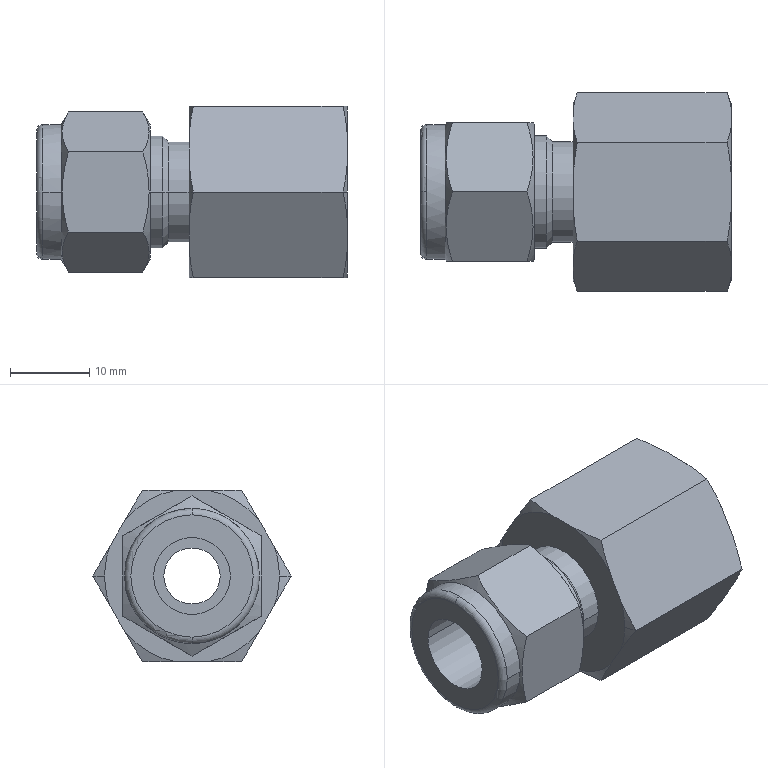Part | STEP file | FITTING-UNION-10Ax10A | 1 solid | 57 faces | box 39.153 x 25 x 21.651 mm | volume 8100 mm3 | cone 28 | plane 17 | cylinder 10 | torus 2 | commonest cylinder face diameters 7.1 x2 9.67 x2 12.65 x2 14.152 x2 17 x2